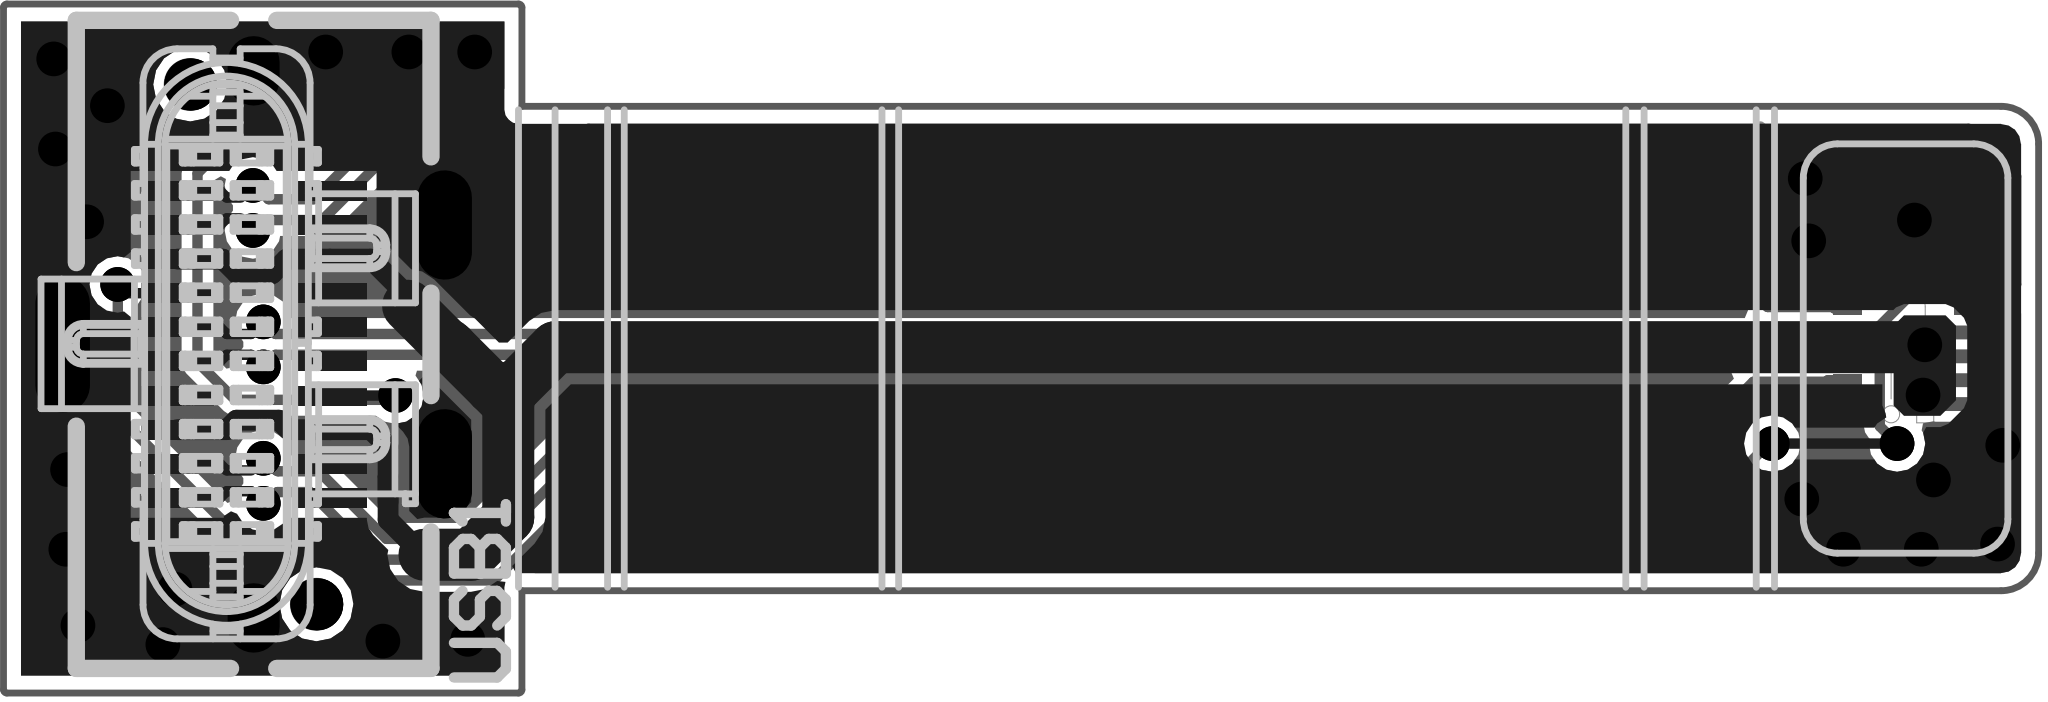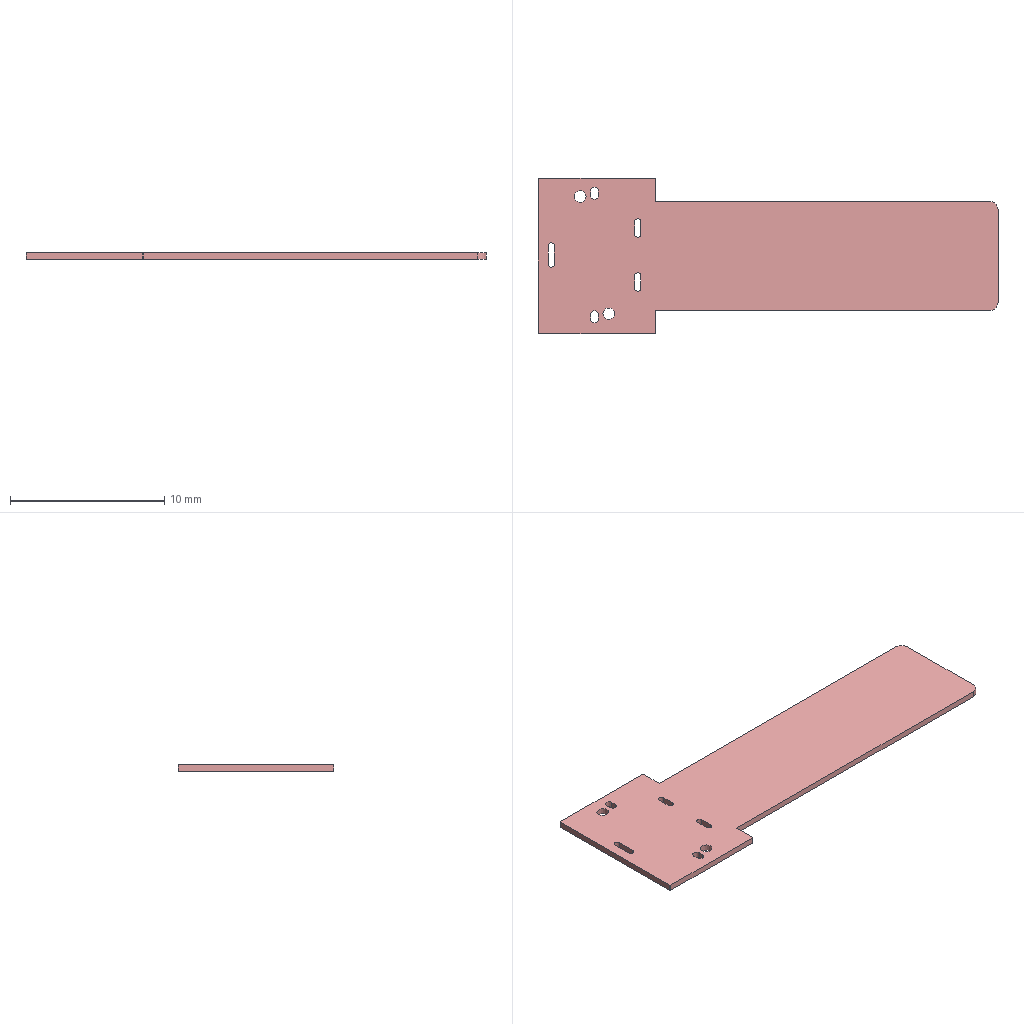Circuit board layout | Altium Designer | box 29.8 x 10.1 x 0.4 mm
Layer stack:
# Altium Designer layer stack of 10 (unit mm; dielectric type: 0 none, 1 core, 2 prepreg, 3 surface material)
index,name,kind,layer,copper_thickness_mm,dielectric_type,dielectric_thickness_mm,dielectric_material,dielectric_constant
0,Top Paste Mask Layer,other,,,,,,
1,Top Silkscreen Layer,other,,,,,,
2,Top Solder Mask Layer,dielectric,,,3,0.0102,Solder Resist,3.5
3,Top Layer,copper,Top Layer,0.0356,,,,
4,Dielectric1,dielectric,,,1,0.32,FR-4,4.8
5,POWER,copper,POWER,0.0356,,,,
6,Dielectric5,dielectric,,,2,0.32,FR-4,4.8
7,GND,copper,GND,0.0356,,,,
8,Dielectric6,dielectric,,,1,0.32,FR-4,4.8
9,Bottom Layer,copper,Bottom Layer,0.0356,,,,
10,Bottom Solder Mask Layer,dielectric,,,3,0.0102,Solder Resist,3.5
11,Bottom Silkscreen Layer,other,,,,,,
12,Bottom Paste Mask Layer,other,,,,,,
# drill layer pairs: low layer,high layer
drill_pair,Top Layer,Bottom Layer
Part placement:
Designator,Comment,Layer,Footprint,Center-X(mm),Center-Y(mm),Rotation
J1,BK13C06-16DS,BottomLayer,BK13C06-16DS_AA,110.424,87.611,90
USB1,TYPEC-952-ACP24,TopLayer,USB-C-SMD_TYPEC-952-ACP24,86.167,87.611,270
Pad and via stacks:
# Altium Designer via and pad stacks of 10 (unit mm). Each distinct definition once, with the count of objects using it.
# via: kind,start_layer,end_layer,hole_mm,diameter_mm,mode(0 simple;1 top-mid-bottom;2 full stack),diameter_per_layer,count,example_net
# pad: kind,layer,hole_mm,hole_type(0 round;1 square;2 slot),plating,top_size,top_shape(1 round;2 rect;3 octagon;9 rounded rect),mid_size,bottom_size,mode,footprint,size_per_layer,count,example
pad,Top Layer,0,0,plated,0.9x0.2,2,0.9x0.2,0.9x0.2,0,CONN-SMD_34P-P0.35_BAF92-34073-0508,,2,J1.40
pad,Top Layer,0,0,plated,0.45x0.3,2,0.45x0.3,0.45x0.3,0,CONN-SMD_34P-P0.35_BAF92-34073-0508,,4,J1.36
pad,Top Layer,0,0,plated,0.13x0.6,2,0.13x0.6,0.13x0.6,0,CONN-SMD_34P-P0.35_BAF92-34073-0508,,34,J1.18
pad,Top Layer,0,0,plated,0.4999x0.2,2,0.4999x0.2,0.4999x0.2,0,CONN-SMD_KYOCERA-AVX_145804030020829,,30,J2.10
via,Top Layer,Bottom Layer,0.2032,0.4064,0,,86,AGND
Copper pours:
name,layer,net,type(0 solid;1 hatched;2 none)
Bottom Layer-No Net,Top Layer,AGND,0
Bottom Layer-No Net,Top Layer,VDD_3V3,0
Bottom Layer-No Net,Bottom Layer,AGND,0
Design rules, without the lines most boards share:
# Altium Designer design rules of 10 (exported by Altium Designer, unit mm)
# columns: name | kind | enabled | priority | scope1 | scope2 | descriptor | typed fields (field=value)
Clearance_1 | 0 | enabled | 1 | inpolygon | All | Clearance Constraint (Gap=8mil) (inpolygon),(All) | gap=0.2032
Clearance | 0 | enabled | 2 | All | All | Clearance Constraint (Gap=5mil) (All),(All) | gap=0.127
PlaneConnect | 6 | enabled | 1 | All | All | Power Plane Connect Rule(Direct Connect )(Expansion=20mil) (Conductor Width=10mil) (Air Gap=10mil) (Entries=4) (All) | relief_conductor_width=0.254 relief_entries=4 relief_expansion=0.508
PlaneClearance | 12 | enabled | 1 | All | All | Power Plane Clearance (Clearance =6mil) (All) | clearance=0.1524
PolygonConnect | 20 | enabled | 1 | All | All | Polygon Connect Rule(Direct Connect )(Conductor Width=10mil) (Relief Angle=90 Angle) (Entries=4) (Air Gap Width=10mil) (All),(All) | connect_style(0=relief,1=direct,2=none)=1 relief_conductor_width=0.254 relief_entries=4
Width | 2 | enabled | 1 | All | All | Width Constraint (Min=5mil) (Max=40mil) (Preferred=5mil) (All) |
RoutingVias | 11 | enabled | 1 | All | All | Routing Via (MinHoleWidth=8mil) (MaxHoleWidth=8mil) (PreferredHoleWidth=8mil) (MinWidth=16mil) (MaxWidth=16mil) (PreferedWidth=16mil) (All) | via_min_hole=0.2032 via_max_hole=0.2032 via_preferred_diameter=0.4064 via_preferred_hole=0.2032
PasteMaskExpansion | 14 | enabled | 1 | All | All | Paste Mask Expansion (Expansion =0mil) (All) | expansion=0
SolderMaskExpansion | 13 | enabled | 1 | All | All | Solder Mask Expansion (Expansion =4mil) (All) | expansion=0.1016
HoleSize | 42 | enabled | 1 | All | All | Hole Size Constraint (Min=1mil) (Max=500mil) (All) |
DiffPairsRouting | 51 | enabled | 1 | All | All | Differential Pairs Uncoupled Length using the Gap Constraints (Min=5mil) (Max=5mil) (Prefered=5mil)  and Width Constraints (Min=15mil) (Max=15mil) (Prefered=15mil) (All) |
HoleToHoleClearance | 52 | enabled | 1 | All | All | Hole To Hole Clearance (Gap=0mil) (All),(All) | gap=0
MinimumSolderMaskSliver | 53 | enabled | 1 | All | All | Minimum Solder Mask Sliver (Gap=0mil) (All),(All) |
SilkscreenOverComponentPads | 54 | enabled | 1 | IsPad | All | Silk To Solder Mask (Clearance=0mil) (IsPad),(All) |
SilkToSilkClearance | 55 | enabled | 1 | All | All | Silk to Silk (Clearance=0mil) (All),(All) |
Classes set for this board:
# Altium Designer classes of 10 (member kind: 0 net, 1 component, 2 from-to, 3 pad, 4 layer, 5 differential pair, 6 design channel, 7 polygon, 8 structure, 9 xSignal)
# columns: class name | member kind | superclass | members
1_P1.schdoc | 1 | no | J1; J2;